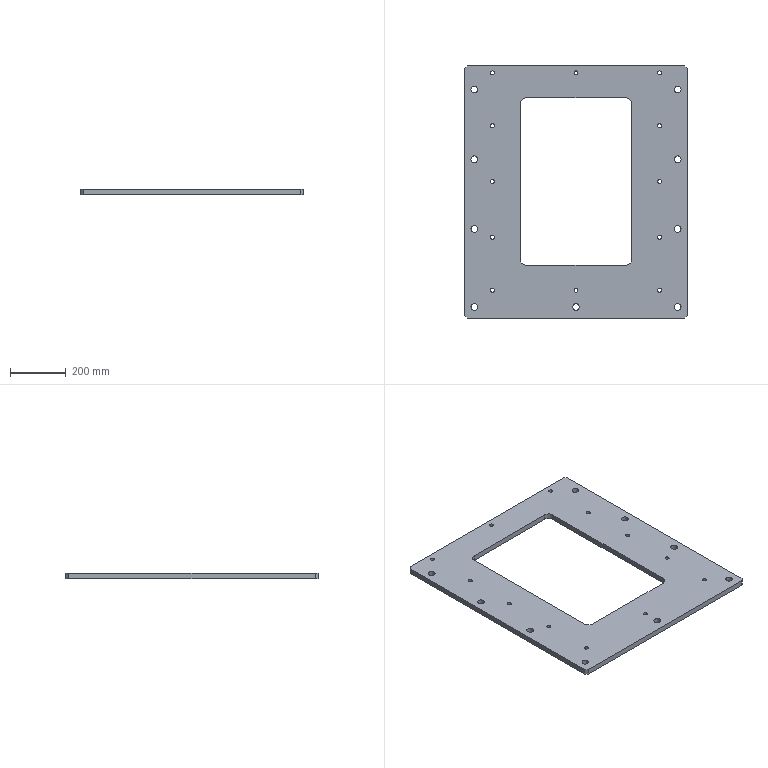Part | SolidWorks | features HoleWzd 2, ICE 2, Chamfer 1, Extrusion 1, Fillet 1 | 1 solid | 60 faces | box 800 x 905 x 20 mm | volume 9564492 mm3 | cylinder 46 | plane 14 | commonest cylinder face diameters 14 x24 24 x18 40 x4